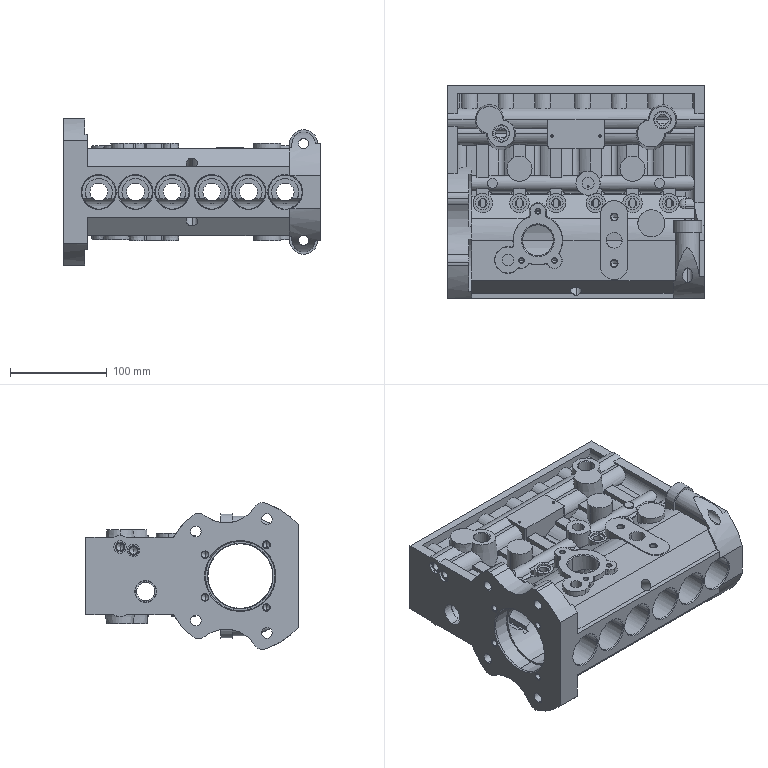Part | SolidWorks | features BaseBody 1 | 1 solid | 1095 faces | box 266 x 220 x 152.149 mm | volume 2615016 mm3 | cylinder 522 | plane 301 | cone 266 | sphere 4 | torus 2 | commonest cylinder face diameters 20 x46 52 x40 35 x30 28 x27 12.5 x26 10.2 x24